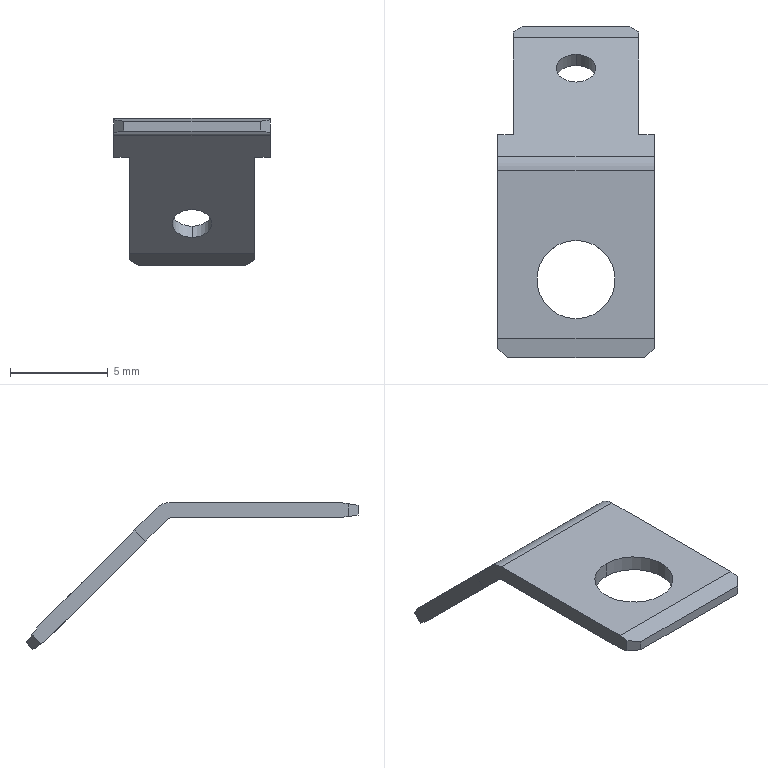Part | STEP file | DXDZ_1_1_1_1 | 1 solid | 26 faces | box 8 x 16.965 x 7.531 mm | volume 100.473 mm3 | plane 20 | cylinder 6 | commonest cylinder face diameters 2 x3 4 x2 0.4 x1
STEP:
#1=CARTESIAN_POINT('',(0.,0.,0.));
#2=DIRECTION('',(0.,0.,1.));
#3=DIRECTION('',(1.,0.,0.));
#4=AXIS2_PLACEMENT_3D('',#1,#2,#3);
#5=CARTESIAN_POINT('',(0.,0.8485,-1.98));
#6=VERTEX_POINT('',#5);
#7=CARTESIAN_POINT('',(0.,1.414,-1.414));
#8=VERTEX_POINT('',#7);
#9=CARTESIAN_POINT('',(0.,0.8485,-1.98));
#10=DIRECTION('',(0.,0.7071,0.7071));
#11=VECTOR('',#10,0.8);
#12=LINE('',#9,#11);
#13=EDGE_CURVE('',#6,#8,#12,.T.);
#14=ORIENTED_EDGE('',*,*,#13,.T.);
#15=CARTESIAN_POINT('',(0.,0.2929,-0.2929));
#16=VERTEX_POINT('',#15);
#17=CARTESIAN_POINT('',(0.,1.414,-1.414));
#18=DIRECTION('',(0.,-0.7071,0.7071));
#19=VECTOR('',#18,1.586);
#20=LINE('',#17,#19);
#21=EDGE_CURVE('',#8,#16,#20,.T.);
#22=ORIENTED_EDGE('',*,*,#21,.T.);
#23=CARTESIAN_POINT('',(0.,-0.4142,0.));
#24=VERTEX_POINT('',#23);
#25=CARTESIAN_POINT('',(0.,-0.4142,-1.));
#26=DIRECTION('',(1.,0.,0.));
#27=DIRECTION('',(0.,0.7071,0.7071));
#28=AXIS2_PLACEMENT_3D('',#25,#26,#27);
#29=CIRCLE('',#28,1.);
#30=EDGE_CURVE('',#16,#24,#29,.T.);
#31=ORIENTED_EDGE('',*,*,#30,.T.);
#32=CARTESIAN_POINT('',(0.,-9.,0.));
#33=VERTEX_POINT('',#32);
#34=CARTESIAN_POINT('',(0.,-0.4142,0.));
#35=DIRECTION('',(0.,-1.,0.));
#36=VECTOR('',#35,8.586);
#37=LINE('',#34,#36);
#38=EDGE_CURVE('',#24,#33,#37,.T.);
#39=ORIENTED_EDGE('',*,*,#38,.T.);
#40=CARTESIAN_POINT('',(0.,-9.5,-0.075));
#41=VERTEX_POINT('',#40);
#42=CARTESIAN_POINT('',(0.,-9.,0.));
#43=DIRECTION('',(0.,-0.9889,-0.1483));
#44=VECTOR('',#43,0.5056);
#45=LINE('',#42,#44);
#46=EDGE_CURVE('',#33,#41,#45,.T.);
#47=ORIENTED_EDGE('',*,*,#46,.T.);
#48=CARTESIAN_POINT('',(0.,-9.5,-0.725));
#49=VERTEX_POINT('',#48);
#50=CARTESIAN_POINT('',(0.,-9.5,-0.725));
#51=DIRECTION('',(0.,0.,1.));
#52=VECTOR('',#51,0.65);
#53=LINE('',#50,#52);
#54=EDGE_CURVE('',#49,#41,#53,.T.);
#55=ORIENTED_EDGE('',*,*,#54,.F.);
#56=CARTESIAN_POINT('',(0.,-9.,-0.8));
#57=VERTEX_POINT('',#56);
#58=CARTESIAN_POINT('',(0.,-9.5,-0.725));
#59=DIRECTION('',(0.,0.9889,-0.1483));
#60=VECTOR('',#59,0.5056);
#61=LINE('',#58,#60);
#62=EDGE_CURVE('',#49,#57,#61,.T.);
#63=ORIENTED_EDGE('',*,*,#62,.T.);
#64=CARTESIAN_POINT('',(0.,-0.4142,-0.8));
#65=VERTEX_POINT('',#64);
#66=CARTESIAN_POINT('',(0.,-9.,-0.8));
#67=DIRECTION('',(0.,1.,0.));
#68=VECTOR('',#67,8.586);
#69=LINE('',#66,#68);
#70=EDGE_CURVE('',#57,#65,#69,.T.);
#71=ORIENTED_EDGE('',*,*,#70,.T.);
#72=CARTESIAN_POINT('',(0.,-0.2728,-0.8586));
#73=VERTEX_POINT('',#72);
#74=CARTESIAN_POINT('',(0.,-0.4142,-1.));
#75=DIRECTION('',(-1.,0.,0.));
#76=DIRECTION('',(0.,0.,1.));
#77=AXIS2_PLACEMENT_3D('',#74,#75,#76);
#78=CIRCLE('',#77,0.2);
#79=EDGE_CURVE('',#65,#73,#78,.T.);
#80=ORIENTED_EDGE('',*,*,#79,.T.);
#81=CARTESIAN_POINT('',(0.,-0.2728,-0.8586));
#82=DIRECTION('',(0.,0.7071,-0.7071));
#83=VECTOR('',#82,1.586);
#84=LINE('',#81,#83);
#85=EDGE_CURVE('',#73,#6,#84,.T.);
#86=ORIENTED_EDGE('',*,*,#85,.T.);
#87=EDGE_LOOP('',(#14,#22,#31,#39,#47,#55,#63,#71,#80,#86));
#88=FACE_OUTER_BOUND('',#87,.F.);
#89=CARTESIAN_POINT('',(0.,0.,0.));
#90=DIRECTION('',(1.,0.,0.));
#91=DIRECTION('',(0.,-1.,0.));
#92=AXIS2_PLACEMENT_3D('',#89,#90,#91);
#93=PLANE('',#92);
#94=ADVANCED_FACE('',(#88),#93,.F.);
#95=ORIENTED_EDGE('',*,*,#13,.F.);
#96=CARTESIAN_POINT('',(0.8,0.8485,-1.98));
#97=VERTEX_POINT('',#96);
#98=CARTESIAN_POINT('',(0.,0.8485,-1.98));
#99=DIRECTION('',(1.,0.,0.));
#100=VECTOR('',#99,0.8);
#101=LINE('',#98,#100);
#102=EDGE_CURVE('',#6,#97,#101,.T.);
#103=ORIENTED_EDGE('',*,*,#102,.T.);
#104=CARTESIAN_POINT('',(0.8,1.414,-1.414));
#105=VERTEX_POINT('',#104);
#106=CARTESIAN_POINT('',(0.8,0.8485,-1.98));
#107=DIRECTION('',(0.,0.7071,0.7071));
#108=VECTOR('',#107,0.8);
#109=LINE('',#106,#108);
#110=EDGE_CURVE('',#97,#105,#109,.T.);
#111=ORIENTED_EDGE('',*,*,#110,.T.);
#112=CARTESIAN_POINT('',(0.,1.414,-1.414));
#113=DIRECTION('',(1.,0.,0.));
#114=VECTOR('',#113,0.8);
#115=LINE('',#112,#114);
#116=EDGE_CURVE('',#8,#105,#115,.T.);
#117=ORIENTED_EDGE('',*,*,#116,.F.);
#118=EDGE_LOOP('',(#95,#103,#111,#117));
#119=FACE_OUTER_BOUND('',#118,.F.);
#120=CARTESIAN_POINT('',(0.8,0.8485,-1.98));
#121=DIRECTION('',(0.,-0.7071,0.7071));
#122=DIRECTION('',(-1.,0.,0.));
#123=AXIS2_PLACEMENT_3D('',#120,#121,#122);
#124=PLANE('',#123);
#125=ADVANCED_FACE('',(#119),#124,.F.);
#126=CARTESIAN_POINT('',(7.2,5.798,-6.93));
#127=VERTEX_POINT('',#126);
#128=CARTESIAN_POINT('',(0.8,5.798,-6.93));
#129=VERTEX_POINT('',#128);
#130=CARTESIAN_POINT('',(7.2,5.798,-6.93));
#131=DIRECTION('',(-1.,0.,0.));
#132=VECTOR('',#131,6.4);
#133=LINE('',#130,#132);
#134=EDGE_CURVE('',#127,#129,#133,.T.);
#135=ORIENTED_EDGE('',*,*,#134,.T.);
#136=CARTESIAN_POINT('',(0.8,5.798,-6.93));
#137=DIRECTION('',(0.,-0.7071,0.7071));
#138=VECTOR('',#137,7.);
#139=LINE('',#136,#138);
#140=EDGE_CURVE('',#129,#97,#139,.T.);
#141=ORIENTED_EDGE('',*,*,#140,.T.);
#142=ORIENTED_EDGE('',*,*,#102,.F.);
#143=ORIENTED_EDGE('',*,*,#85,.F.);
#144=CARTESIAN_POINT('',(8.,-0.2728,-0.8586));
#145=VERTEX_POINT('',#144);
#146=CARTESIAN_POINT('',(8.,-0.2728,-0.8586));
#147=DIRECTION('',(-1.,0.,0.));
#148=VECTOR('',#147,8.);
#149=LINE('',#146,#148);
#150=EDGE_CURVE('',#145,#73,#149,.T.);
#151=ORIENTED_EDGE('',*,*,#150,.F.);
#152=CARTESIAN_POINT('',(8.,0.8485,-1.98));
#153=VERTEX_POINT('',#152);
#154=CARTESIAN_POINT('',(8.,0.8485,-1.98));
#155=DIRECTION('',(0.,-0.7071,0.7071));
#156=VECTOR('',#155,1.586);
#157=LINE('',#154,#156);
#158=EDGE_CURVE('',#153,#145,#157,.T.);
#159=ORIENTED_EDGE('',*,*,#158,.F.);
#160=CARTESIAN_POINT('',(7.2,0.8485,-1.98));
#161=VERTEX_POINT('',#160);
#162=CARTESIAN_POINT('',(8.,0.8485,-1.98));
#163=DIRECTION('',(-1.,0.,0.));
#164=VECTOR('',#163,0.8);
#165=LINE('',#162,#164);
#166=EDGE_CURVE('',#153,#161,#165,.T.);
#167=ORIENTED_EDGE('',*,*,#166,.T.);
#168=CARTESIAN_POINT('',(7.2,5.798,-6.93));
#169=DIRECTION('',(0.,-0.7071,0.7071));
#170=VECTOR('',#169,7.);
#171=LINE('',#168,#170);
#172=EDGE_CURVE('',#127,#161,#171,.T.);
#173=ORIENTED_EDGE('',*,*,#172,.F.);
#174=EDGE_LOOP('',(#135,#141,#142,#143,#151,#159,#167,#173));
#175=FACE_OUTER_BOUND('',#174,.F.);
#176=CARTESIAN_POINT('',(4.,3.536,-4.667));
#177=VERTEX_POINT('',#176);
#178=CARTESIAN_POINT('',(4.,4.95,-6.081));
#179=VERTEX_POINT('',#178);
#180=CARTESIAN_POINT('',(4.,4.243,-5.374));
#181=DIRECTION('',(0.,-0.7071,-0.7071));
#182=DIRECTION('',(0.,-0.7071,0.7071));
#183=AXIS2_PLACEMENT_3D('',#180,#181,#182);
#184=CIRCLE('',#183,1.);
#185=EDGE_CURVE('',#177,#179,#184,.T.);
#186=ORIENTED_EDGE('',*,*,#185,.T.);
#187=CARTESIAN_POINT('',(4.,4.243,-5.374));
#188=DIRECTION('',(0.,-0.7071,-0.7071));
#189=DIRECTION('',(0.,0.7071,-0.7071));
#190=AXIS2_PLACEMENT_3D('',#187,#188,#189);
#191=CIRCLE('',#190,1.);
#192=EDGE_CURVE('',#179,#177,#191,.T.);
#193=ORIENTED_EDGE('',*,*,#192,.T.);
#194=EDGE_LOOP('',(#186,#193));
#195=FACE_BOUND('',#194,.F.);
#196=CARTESIAN_POINT('',(0.,-0.3314,-0.8));
#197=DIRECTION('',(0.,-0.7071,-0.7071));
#198=DIRECTION('',(0.,0.7071,-0.7071));
#199=AXIS2_PLACEMENT_3D('',#196,#197,#198);
#200=PLANE('',#199);
#201=ADVANCED_FACE('',(#175,#195),#200,.T.);
#202=CARTESIAN_POINT('',(1.3,6.611,-7.531));
#203=VERTEX_POINT('',#202);
#204=CARTESIAN_POINT('',(0.8,6.205,-7.23));
#205=VERTEX_POINT('',#204);
#206=CARTESIAN_POINT('',(1.3,6.611,-7.531));
#207=DIRECTION('',(-0.7032,-0.5718,0.4226));
#208=VECTOR('',#207,0.7111);
#209=LINE('',#206,#208);
#210=EDGE_CURVE('',#203,#205,#209,.T.);
#211=ORIENTED_EDGE('',*,*,#210,.T.);
#212=CARTESIAN_POINT('',(0.8,5.798,-6.93));
#213=DIRECTION('',(0.,0.8042,-0.5944));
#214=VECTOR('',#213,0.5056);
#215=LINE('',#212,#214);
#216=EDGE_CURVE('',#129,#205,#215,.T.);
#217=ORIENTED_EDGE('',*,*,#216,.F.);
#218=ORIENTED_EDGE('',*,*,#134,.F.);
#219=CARTESIAN_POINT('',(7.2,6.205,-7.23));
#220=VERTEX_POINT('',#219);
#221=CARTESIAN_POINT('',(7.2,6.205,-7.23));
#222=DIRECTION('',(0.,-0.8042,0.5944));
#223=VECTOR('',#222,0.5056);
#224=LINE('',#221,#223);
#225=EDGE_CURVE('',#220,#127,#224,.T.);
#226=ORIENTED_EDGE('',*,*,#225,.F.);
#227=CARTESIAN_POINT('',(6.7,6.611,-7.531));
#228=VERTEX_POINT('',#227);
#229=CARTESIAN_POINT('',(7.2,6.205,-7.23));
#230=DIRECTION('',(-0.7032,0.5718,-0.4226));
#231=VECTOR('',#230,0.7111);
#232=LINE('',#229,#231);
#233=EDGE_CURVE('',#220,#228,#232,.T.);
#234=ORIENTED_EDGE('',*,*,#233,.T.);
#235=CARTESIAN_POINT('',(6.7,6.611,-7.531));
#236=DIRECTION('',(-1.,0.,0.));
#237=VECTOR('',#236,5.4);
#238=LINE('',#235,#237);
#239=EDGE_CURVE('',#228,#203,#238,.T.);
#240=ORIENTED_EDGE('',*,*,#239,.T.);
#241=EDGE_LOOP('',(#211,#217,#218,#226,#234,#240));
#242=FACE_OUTER_BOUND('',#241,.F.);
#243=CARTESIAN_POINT('',(4.,6.205,-7.23));
#244=DIRECTION('',(0.,-0.5944,-0.8042));
#245=DIRECTION('',(0.,-0.8042,0.5944));
#246=AXIS2_PLACEMENT_3D('',#243,#244,#245);
#247=PLANE('',#246);
#248=ADVANCED_FACE('',(#242),#247,.T.);
#249=CARTESIAN_POINT('',(0.8,6.664,-6.771));
#250=VERTEX_POINT('',#249);
#251=CARTESIAN_POINT('',(1.3,6.965,-7.177));
#252=VERTEX_POINT('',#251);
#253=CARTESIAN_POINT('',(0.8,6.664,-6.771));
#254=DIRECTION('',(0.7032,0.4226,-0.5718));
#255=VECTOR('',#254,0.7111);
#256=LINE('',#253,#255);
#257=EDGE_CURVE('',#250,#252,#256,.T.);
#258=ORIENTED_EDGE('',*,*,#257,.F.);
#259=CARTESIAN_POINT('',(0.8,6.205,-7.23));
#260=DIRECTION('',(0.,0.7071,0.7071));
#261=VECTOR('',#260,0.65);
#262=LINE('',#259,#261);
#263=EDGE_CURVE('',#205,#250,#262,.T.);
#264=ORIENTED_EDGE('',*,*,#263,.F.);
#265=ORIENTED_EDGE('',*,*,#210,.F.);
#266=CARTESIAN_POINT('',(1.3,6.611,-7.531));
#267=DIRECTION('',(0.,0.7071,0.7071));
#268=VECTOR('',#267,0.5);
#269=LINE('',#266,#268);
#270=EDGE_CURVE('',#203,#252,#269,.T.);
#271=ORIENTED_EDGE('',*,*,#270,.T.);
#272=EDGE_LOOP('',(#258,#264,#265,#271));
#273=FACE_OUTER_BOUND('',#272,.F.);
#274=CARTESIAN_POINT('',(1.05,6.611,-7.177));
#275=DIRECTION('',(-0.7071,0.5,-0.5));
#276=DIRECTION('',(-0.7071,-0.5,0.5));
#277=AXIS2_PLACEMENT_3D('',#274,#275,#276);
#278=PLANE('',#277);
#279=ADVANCED_FACE('',(#273),#278,.T.);
#280=CARTESIAN_POINT('',(0.8,6.364,-6.364));
#281=VERTEX_POINT('',#280);
#282=CARTESIAN_POINT('',(0.8,6.664,-6.771));
#283=DIRECTION('',(0.,-0.5944,0.8042));
#284=VECTOR('',#283,0.5056);
#285=LINE('',#282,#284);
#286=EDGE_CURVE('',#250,#281,#285,.T.);
#287=ORIENTED_EDGE('',*,*,#286,.F.);
#288=ORIENTED_EDGE('',*,*,#257,.T.);
#289=CARTESIAN_POINT('',(6.7,6.965,-7.177));
#290=VERTEX_POINT('',#289);
#291=CARTESIAN_POINT('',(6.7,6.965,-7.177));
#292=DIRECTION('',(-1.,0.,0.));
#293=VECTOR('',#292,5.4);
#294=LINE('',#291,#293);
#295=EDGE_CURVE('',#290,#252,#294,.T.);
#296=ORIENTED_EDGE('',*,*,#295,.F.);
#297=CARTESIAN_POINT('',(7.2,6.664,-6.771));
#298=VERTEX_POINT('',#297);
#299=CARTESIAN_POINT('',(6.7,6.965,-7.177));
#300=DIRECTION('',(0.7032,-0.4226,0.5718));
#301=VECTOR('',#300,0.7111);
#302=LINE('',#299,#301);
#303=EDGE_CURVE('',#290,#298,#302,.T.);
#304=ORIENTED_EDGE('',*,*,#303,.T.);
#305=CARTESIAN_POINT('',(7.2,6.364,-6.364));
#306=VERTEX_POINT('',#305);
#307=CARTESIAN_POINT('',(7.2,6.364,-6.364));
#308=DIRECTION('',(0.,0.5944,-0.8042));
#309=VECTOR('',#308,0.5056);
#310=LINE('',#307,#309);
#311=EDGE_CURVE('',#306,#298,#310,.T.);
#312=ORIENTED_EDGE('',*,*,#311,.F.);
#313=CARTESIAN_POINT('',(7.2,6.364,-6.364));
#314=DIRECTION('',(-1.,0.,0.));
#315=VECTOR('',#314,6.4);
#316=LINE('',#313,#315);
#317=EDGE_CURVE('',#306,#281,#316,.T.);
#318=ORIENTED_EDGE('',*,*,#317,.T.);
#319=EDGE_LOOP('',(#287,#288,#296,#304,#312,#318));
#320=FACE_OUTER_BOUND('',#319,.F.);
#321=CARTESIAN_POINT('',(4.,6.664,-6.771));
#322=DIRECTION('',(0.,0.8042,0.5944));
#323=DIRECTION('',(0.,0.5944,-0.8042));
#324=AXIS2_PLACEMENT_3D('',#321,#322,#323);
#325=PLANE('',#324);
#326=ADVANCED_FACE('',(#320),#325,.T.);
#327=ORIENTED_EDGE('',*,*,#286,.T.);
#328=CARTESIAN_POINT('',(0.8,6.364,-6.364));
#329=DIRECTION('',(0.,-0.7071,0.7071));
#330=VECTOR('',#329,7.);
#331=LINE('',#328,#330);
#332=EDGE_CURVE('',#281,#105,#331,.T.);
#333=ORIENTED_EDGE('',*,*,#332,.T.);
#334=ORIENTED_EDGE('',*,*,#110,.F.);
#335=ORIENTED_EDGE('',*,*,#140,.F.);
#336=ORIENTED_EDGE('',*,*,#216,.T.);
#337=ORIENTED_EDGE('',*,*,#263,.T.);
#338=EDGE_LOOP('',(#327,#333,#334,#335,#336,#337));
#339=FACE_OUTER_BOUND('',#338,.F.);
#340=CARTESIAN_POINT('',(0.8,6.505,-7.637));
#341=DIRECTION('',(1.,0.,0.));
#342=DIRECTION('',(0.,-0.7071,0.7071));
#343=AXIS2_PLACEMENT_3D('',#340,#341,#342);
#344=PLANE('',#343);
#345=ADVANCED_FACE('',(#339),#344,.F.);
#346=ORIENTED_EDGE('',*,*,#317,.F.);
#347=CARTESIAN_POINT('',(7.2,1.414,-1.414));
#348=VERTEX_POINT('',#347);
#349=CARTESIAN_POINT('',(7.2,6.364,-6.364));
#350=DIRECTION('',(0.,-0.7071,0.7071));
#351=VECTOR('',#350,7.);
#352=LINE('',#349,#351);
#353=EDGE_CURVE('',#306,#348,#352,.T.);
#354=ORIENTED_EDGE('',*,*,#353,.T.);
#355=CARTESIAN_POINT('',(8.,1.414,-1.414));
#356=VERTEX_POINT('',#355);
#357=CARTESIAN_POINT('',(8.,1.414,-1.414));
#358=DIRECTION('',(-1.,0.,0.));
#359=VECTOR('',#358,0.8);
#360=LINE('',#357,#359);
#361=EDGE_CURVE('',#356,#348,#360,.T.);
#362=ORIENTED_EDGE('',*,*,#361,.F.);
#363=CARTESIAN_POINT('',(8.,0.2929,-0.2929));
#364=VERTEX_POINT('',#363);
#365=CARTESIAN_POINT('',(8.,0.2929,-0.2929));
#366=DIRECTION('',(0.,0.7071,-0.7071));
#367=VECTOR('',#366,1.586);
#368=LINE('',#365,#367);
#369=EDGE_CURVE('',#364,#356,#368,.T.);
#370=ORIENTED_EDGE('',*,*,#369,.F.);
#371=CARTESIAN_POINT('',(0.,0.2929,-0.2929));
#372=DIRECTION('',(1.,0.,0.));
#373=VECTOR('',#372,8.);
#374=LINE('',#371,#373);
#375=EDGE_CURVE('',#16,#364,#374,.T.);
#376=ORIENTED_EDGE('',*,*,#375,.F.);
#377=ORIENTED_EDGE('',*,*,#21,.F.);
#378=ORIENTED_EDGE('',*,*,#116,.T.);
#379=ORIENTED_EDGE('',*,*,#332,.F.);
#380=EDGE_LOOP('',(#346,#354,#362,#370,#376,#377,#378,#379));
#381=FACE_OUTER_BOUND('',#380,.F.);
#382=CARTESIAN_POINT('',(4.,5.515,-5.515));
#383=VERTEX_POINT('',#382);
#384=CARTESIAN_POINT('',(4.,4.101,-4.101));
#385=VERTEX_POINT('',#384);
#386=CARTESIAN_POINT('',(4.,4.808,-4.808));
#387=DIRECTION('',(0.,0.7071,0.7071));
#388=DIRECTION('',(0.,0.7071,-0.7071));
#389=AXIS2_PLACEMENT_3D('',#386,#387,#388);
#390=CIRCLE('',#389,1.);
#391=EDGE_CURVE('',#383,#385,#390,.T.);
#392=ORIENTED_EDGE('',*,*,#391,.T.);
#393=CARTESIAN_POINT('',(4.,4.808,-4.808));
#394=DIRECTION('',(0.,0.7071,0.7071));
#395=DIRECTION('',(0.,-0.7071,0.7071));
#396=AXIS2_PLACEMENT_3D('',#393,#394,#395);
#397=CIRCLE('',#396,1.);
#398=EDGE_CURVE('',#385,#383,#397,.T.);
#399=ORIENTED_EDGE('',*,*,#398,.T.);
#400=EDGE_LOOP('',(#392,#399));
#401=FACE_BOUND('',#400,.F.);
#402=CARTESIAN_POINT('',(0.,7.071,-7.071));
#403=DIRECTION('',(0.,0.7071,0.7071));
#404=DIRECTION('',(0.,-0.7071,0.7071));
#405=AXIS2_PLACEMENT_3D('',#402,#403,#404);
#406=PLANE('',#405);
#407=ADVANCED_FACE('',(#381,#401),#406,.T.);
#408=ORIENTED_EDGE('',*,*,#311,.T.);
#409=CARTESIAN_POINT('',(7.2,6.664,-6.771));
#410=DIRECTION('',(0.,-0.7071,-0.7071));
#411=VECTOR('',#410,0.65);
#412=LINE('',#409,#411);
#413=EDGE_CURVE('',#298,#220,#412,.T.);
#414=ORIENTED_EDGE('',*,*,#413,.T.);
#415=ORIENTED_EDGE('',*,*,#225,.T.);
#416=ORIENTED_EDGE('',*,*,#172,.T.);
#417=CARTESIAN_POINT('',(7.2,0.8485,-1.98));
#418=DIRECTION('',(0.,0.7071,0.7071));
#419=VECTOR('',#418,0.8);
#420=LINE('',#417,#419);
#421=EDGE_CURVE('',#161,#348,#420,.T.);
#422=ORIENTED_EDGE('',*,*,#421,.T.);
#423=ORIENTED_EDGE('',*,*,#353,.F.);
#424=EDGE_LOOP('',(#408,#414,#415,#416,#422,#423));
#425=FACE_OUTER_BOUND('',#424,.F.);
#426=CARTESIAN_POINT('',(7.2,0.8485,-1.98));
#427=DIRECTION('',(-1.,0.,0.));
#428=DIRECTION('',(0.,0.7071,-0.7071));
#429=AXIS2_PLACEMENT_3D('',#426,#427,#428);
#430=PLANE('',#429);
#431=ADVANCED_FACE('',(#425),#430,.F.);
#432=ORIENTED_EDGE('',*,*,#303,.F.);
#433=CARTESIAN_POINT('',(6.7,6.965,-7.177));
#434=DIRECTION('',(0.,-0.7071,-0.7071));
#435=VECTOR('',#434,0.5);
#436=LINE('',#433,#435);
#437=EDGE_CURVE('',#290,#228,#436,.T.);
#438=ORIENTED_EDGE('',*,*,#437,.T.);
#439=ORIENTED_EDGE('',*,*,#233,.F.);
#440=ORIENTED_EDGE('',*,*,#413,.F.);
#441=EDGE_LOOP('',(#432,#438,#439,#440));
#442=FACE_OUTER_BOUND('',#441,.F.);
#443=CARTESIAN_POINT('',(6.95,6.611,-7.177));
#444=DIRECTION('',(0.7071,0.5,-0.5));
#445=DIRECTION('',(0.7071,-0.5,0.5));
#446=AXIS2_PLACEMENT_3D('',#443,#444,#445);
#447=PLANE('',#446);
#448=ADVANCED_FACE('',(#442),#447,.T.);
#449=ORIENTED_EDGE('',*,*,#295,.T.);
#450=ORIENTED_EDGE('',*,*,#270,.F.);
#451=ORIENTED_EDGE('',*,*,#239,.F.);
#452=ORIENTED_EDGE('',*,*,#437,.F.);
#453=EDGE_LOOP('',(#449,#450,#451,#452));
#454=FACE_OUTER_BOUND('',#453,.F.);
#455=CARTESIAN_POINT('',(0.,6.505,-7.637));
#456=DIRECTION('',(0.,0.7071,-0.7071));
#457=DIRECTION('',(0.,0.7071,0.7071));
#458=AXIS2_PLACEMENT_3D('',#455,#456,#457);
#459=PLANE('',#458);
#460=ADVANCED_FACE('',(#454),#459,.T.);
#461=CARTESIAN_POINT('',(8.,1.414,-1.414));
#462=DIRECTION('',(0.,-0.7071,-0.7071));
#463=VECTOR('',#462,0.8);
#464=LINE('',#461,#463);
#465=EDGE_CURVE('',#356,#153,#464,.T.);
#466=ORIENTED_EDGE('',*,*,#465,.F.);
#467=ORIENTED_EDGE('',*,*,#361,.T.);
#468=ORIENTED_EDGE('',*,*,#421,.F.);
#469=ORIENTED_EDGE('',*,*,#166,.F.);
#470=EDGE_LOOP('',(#466,#467,#468,#469));
#471=FACE_OUTER_BOUND('',#470,.F.);
#472=CARTESIAN_POINT('',(8.,0.8485,-1.98));
#473=DIRECTION('',(0.,-0.7071,0.7071));
#474=DIRECTION('',(-1.,0.,0.));
#475=AXIS2_PLACEMENT_3D('',#472,#473,#474);
#476=PLANE('',#475);
#477=ADVANCED_FACE('',(#471),#476,.F.);
#478=ORIENTED_EDGE('',*,*,#465,.T.);
#479=ORIENTED_EDGE('',*,*,#158,.T.);
#480=CARTESIAN_POINT('',(8.,-0.4142,-0.8));
#481=VERTEX_POINT('',#480);
#482=CARTESIAN_POINT('',(8.,-0.4142,-1.));
#483=DIRECTION('',(1.,0.,0.));
#484=DIRECTION('',(0.,0.7071,0.7071));
#485=AXIS2_PLACEMENT_3D('',#482,#483,#484);
#486=CIRCLE('',#485,0.2);
#487=EDGE_CURVE('',#145,#481,#486,.T.);
#488=ORIENTED_EDGE('',*,*,#487,.T.);
#489=CARTESIAN_POINT('',(8.,-9.,-0.8));
#490=VERTEX_POINT('',#489);
#491=CARTESIAN_POINT('',(8.,-9.,-0.8));
#492=DIRECTION('',(0.,1.,0.));
#493=VECTOR('',#492,8.586);
#494=LINE('',#491,#493);
#495=EDGE_CURVE('',#490,#481,#494,.T.);
#496=ORIENTED_EDGE('',*,*,#495,.F.);
#497=CARTESIAN_POINT('',(8.,-9.5,-0.725));
#498=VERTEX_POINT('',#497);
#499=CARTESIAN_POINT('',(8.,-9.,-0.8));
#500=DIRECTION('',(0.,-0.9889,0.1483));
#501=VECTOR('',#500,0.5056);
#502=LINE('',#499,#501);
#503=EDGE_CURVE('',#490,#498,#502,.T.);
#504=ORIENTED_EDGE('',*,*,#503,.T.);
#505=CARTESIAN_POINT('',(8.,-9.5,-0.075));
#506=VERTEX_POINT('',#505);
#507=CARTESIAN_POINT('',(8.,-9.5,-0.075));
#508=DIRECTION('',(0.,0.,-1.));
#509=VECTOR('',#508,0.65);
#510=LINE('',#507,#509);
#511=EDGE_CURVE('',#506,#498,#510,.T.);
#512=ORIENTED_EDGE('',*,*,#511,.F.);
#513=CARTESIAN_POINT('',(8.,-9.,0.));
#514=VERTEX_POINT('',#513);
#515=CARTESIAN_POINT('',(8.,-9.5,-0.075));
#516=DIRECTION('',(0.,0.9889,0.1483));
#517=VECTOR('',#516,0.5056);
#518=LINE('',#515,#517);
#519=EDGE_CURVE('',#506,#514,#518,.T.);
#520=ORIENTED_EDGE('',*,*,#519,.T.);
#521=CARTESIAN_POINT('',(8.,-0.4142,0.));
#522=VERTEX_POINT('',#521);
#523=CARTESIAN_POINT('',(8.,-0.4142,0.));
#524=DIRECTION('',(0.,-1.,0.));
#525=VECTOR('',#524,8.586);
#526=LINE('',#523,#525);
#527=EDGE_CURVE('',#522,#514,#526,.T.);
#528=ORIENTED_EDGE('',*,*,#527,.F.);
#529=CARTESIAN_POINT('',(8.,-0.4142,-1.));
#530=DIRECTION('',(-1.,0.,0.));
#531=DIRECTION('',(0.,0.,1.));
#532=AXIS2_PLACEMENT_3D('',#529,#530,#531);
#533=CIRCLE('',#532,1.);
#534=EDGE_CURVE('',#522,#364,#533,.T.);
#535=ORIENTED_EDGE('',*,*,#534,.T.);
#536=ORIENTED_EDGE('',*,*,#369,.T.);
#537=EDGE_LOOP('',(#478,#479,#488,#496,#504,#512,#520,#528,#535,#536));
#538=FACE_OUTER_BOUND('',#537,.F.);
#539=CARTESIAN_POINT('',(8.,0.,0.));
#540=DIRECTION('',(1.,0.,0.));
#541=DIRECTION('',(0.,-1.,0.));
#542=AXIS2_PLACEMENT_3D('',#539,#540,#541);
#543=PLANE('',#542);
#544=ADVANCED_FACE('',(#538),#543,.T.);
#545=ORIENTED_EDGE('',*,*,#150,.T.);
#546=ORIENTED_EDGE('',*,*,#79,.F.);
#547=CARTESIAN_POINT('',(0.,-0.4142,-0.8));
#548=DIRECTION('',(1.,0.,0.));
#549=VECTOR('',#548,8.);
#550=LINE('',#547,#549);
#551=EDGE_CURVE('',#65,#481,#550,.T.);
#552=ORIENTED_EDGE('',*,*,#551,.T.);
#553=ORIENTED_EDGE('',*,*,#487,.F.);
#554=EDGE_LOOP('',(#545,#546,#552,#553));
#555=FACE_OUTER_BOUND('',#554,.F.);
#556=CARTESIAN_POINT('',(-10.429,-0.4142,-1.));
#557=DIRECTION('',(1.,0.,0.));
#558=DIRECTION('',(0.,0.7071,0.7071));
#559=AXIS2_PLACEMENT_3D('',#556,#557,#558);
#560=CYLINDRICAL_SURFACE('',#559,0.2);
#561=ADVANCED_FACE('',(#555),#560,.F.);
#562=CARTESIAN_POINT('',(8.,-9.,-0.8));
#563=DIRECTION('',(-1.,0.,0.));
#564=VECTOR('',#563,8.);
#565=LINE('',#562,#564);
#566=EDGE_CURVE('',#490,#57,#565,.T.);
#567=ORIENTED_EDGE('',*,*,#566,.F.);
#568=ORIENTED_EDGE('',*,*,#495,.T.);
#569=ORIENTED_EDGE('',*,*,#551,.F.);
#570=ORIENTED_EDGE('',*,*,#70,.F.);
#571=EDGE_LOOP('',(#567,#568,#569,#570));
#572=FACE_OUTER_BOUND('',#571,.F.);
#573=CARTESIAN_POINT('',(4.,-8.,-0.8));
#574=VERTEX_POINT('',#573);
#575=CARTESIAN_POINT('',(4.,-4.,-0.8));
#576=VERTEX_POINT('',#575);
#577=CARTESIAN_POINT('',(4.,-6.,-0.8));
#578=DIRECTION('',(0.,0.,-1.));
#579=DIRECTION('',(0.,-1.,0.));
#580=AXIS2_PLACEMENT_3D('',#577,#578,#579);
#581=CIRCLE('',#580,2.);
#582=EDGE_CURVE('',#574,#576,#581,.T.);
#583=ORIENTED_EDGE('',*,*,#582,.T.);
#584=CARTESIAN_POINT('',(4.,-6.,-0.8));
#585=DIRECTION('',(0.,0.,-1.));
#586=DIRECTION('',(0.,1.,0.));
#587=AXIS2_PLACEMENT_3D('',#584,#585,#586);
#588=CIRCLE('',#587,2.);
#589=EDGE_CURVE('',#576,#574,#588,.T.);
#590=ORIENTED_EDGE('',*,*,#589,.T.);
#591=EDGE_LOOP('',(#583,#590));
#592=FACE_BOUND('',#591,.F.);
#593=CARTESIAN_POINT('',(0.,-10.,-0.8));
#594=DIRECTION('',(0.,0.,-1.));
#595=DIRECTION('',(0.,1.,0.));
#596=AXIS2_PLACEMENT_3D('',#593,#594,#595);
#597=PLANE('',#596);
#598=ADVANCED_FACE('',(#572,#592),#597,.T.);
#599=ORIENTED_EDGE('',*,*,#62,.F.);
#600=CARTESIAN_POINT('',(0.5,-10.,-0.65));
#601=VERTEX_POINT('',#600);
#602=CARTESIAN_POINT('',(0.,-9.5,-0.725));
#603=DIRECTION('',(0.7032,-0.7032,0.1055));
#604=VECTOR('',#603,0.7111);
#605=LINE('',#602,#604);
#606=EDGE_CURVE('',#49,#601,#605,.T.);
#607=ORIENTED_EDGE('',*,*,#606,.T.);
#608=CARTESIAN_POINT('',(7.5,-10.,-0.65));
#609=VERTEX_POINT('',#608);
#610=CARTESIAN_POINT('',(7.5,-10.,-0.65));
#611=DIRECTION('',(-1.,0.,0.));
#612=VECTOR('',#611,7.);
#613=LINE('',#610,#612);
#614=EDGE_CURVE('',#609,#601,#613,.T.);
#615=ORIENTED_EDGE('',*,*,#614,.F.);
#616=CARTESIAN_POINT('',(7.5,-10.,-0.65));
#617=DIRECTION('',(0.7032,0.7032,-0.1055));
#618=VECTOR('',#617,0.7111);
#619=LINE('',#616,#618);
#620=EDGE_CURVE('',#609,#498,#619,.T.);
#621=ORIENTED_EDGE('',*,*,#620,.T.);
#622=ORIENTED_EDGE('',*,*,#503,.F.);
#623=ORIENTED_EDGE('',*,*,#566,.T.);
#624=EDGE_LOOP('',(#599,#607,#615,#621,#622,#623));
#625=FACE_OUTER_BOUND('',#624,.F.);
#626=CARTESIAN_POINT('',(4.,-9.5,-0.725));
#627=DIRECTION('',(0.,-0.1483,-0.9889));
#628=DIRECTION('',(0.,-0.9889,0.1483));
#629=AXIS2_PLACEMENT_3D('',#626,#627,#628);
#630=PLANE('',#629);
#631=ADVANCED_FACE('',(#625),#630,.T.);
#632=CARTESIAN_POINT('',(0.5,-10.,-0.15));
#633=VERTEX_POINT('',#632);
#634=CARTESIAN_POINT('',(0.5,-10.,-0.15));
#635=DIRECTION('',(-0.7032,0.7032,0.1055));
#636=VECTOR('',#635,0.7111);
#637=LINE('',#634,#636);
#638=EDGE_CURVE('',#633,#41,#637,.T.);
#639=ORIENTED_EDGE('',*,*,#638,.F.);
#640=CARTESIAN_POINT('',(0.5,-10.,-0.65));
#641=DIRECTION('',(0.,0.,1.));
#642=VECTOR('',#641,0.5);
#643=LINE('',#640,#642);
#644=EDGE_CURVE('',#601,#633,#643,.T.);
#645=ORIENTED_EDGE('',*,*,#644,.F.);
#646=ORIENTED_EDGE('',*,*,#606,.F.);
#647=ORIENTED_EDGE('',*,*,#54,.T.);
#648=EDGE_LOOP('',(#639,#645,#646,#647));
#649=FACE_OUTER_BOUND('',#648,.F.);
#650=CARTESIAN_POINT('',(0.25,-9.75,-0.4));
#651=DIRECTION('',(-0.7071,-0.7071,0.));
#652=DIRECTION('',(0.7071,-0.7071,0.));
#653=AXIS2_PLACEMENT_3D('',#650,#651,#652);
#654=PLANE('',#653);
#655=ADVANCED_FACE('',(#649),#654,.T.);
#656=ORIENTED_EDGE('',*,*,#638,.T.);
#657=ORIENTED_EDGE('',*,*,#46,.F.);
#658=CARTESIAN_POINT('',(8.,-9.,0.));
#659=DIRECTION('',(-1.,0.,0.));
#660=VECTOR('',#659,8.);
#661=LINE('',#658,#660);
#662=EDGE_CURVE('',#514,#33,#661,.T.);
#663=ORIENTED_EDGE('',*,*,#662,.F.);
#664=ORIENTED_EDGE('',*,*,#519,.F.);
#665=CARTESIAN_POINT('',(7.5,-10.,-0.15));
#666=VERTEX_POINT('',#665);
#667=CARTESIAN_POINT('',(8.,-9.5,-0.075));
#668=DIRECTION('',(-0.7032,-0.7032,-0.1055));
#669=VECTOR('',#668,0.7111);
#670=LINE('',#667,#669);
#671=EDGE_CURVE('',#506,#666,#670,.T.);
#672=ORIENTED_EDGE('',*,*,#671,.T.);
#673=CARTESIAN_POINT('',(7.5,-10.,-0.15));
#674=DIRECTION('',(-1.,0.,0.));
#675=VECTOR('',#674,7.);
#676=LINE('',#673,#675);
#677=EDGE_CURVE('',#666,#633,#676,.T.);
#678=ORIENTED_EDGE('',*,*,#677,.T.);
#679=EDGE_LOOP('',(#656,#657,#663,#664,#672,#678));
#680=FACE_OUTER_BOUND('',#679,.F.);
#681=CARTESIAN_POINT('',(4.,-9.5,-0.075));
#682=DIRECTION('',(0.,-0.1483,0.9889));
#683=DIRECTION('',(0.,0.9889,0.1483));
#684=AXIS2_PLACEMENT_3D('',#681,#682,#683);
#685=PLANE('',#684);
#686=ADVANCED_FACE('',(#680),#685,.T.);
#687=ORIENTED_EDGE('',*,*,#662,.T.);
#688=ORIENTED_EDGE('',*,*,#38,.F.);
#689=CARTESIAN_POINT('',(8.,-0.4142,0.));
#690=DIRECTION('',(-1.,0.,0.));
#691=VECTOR('',#690,8.);
#692=LINE('',#689,#691);
#693=EDGE_CURVE('',#522,#24,#692,.T.);
#694=ORIENTED_EDGE('',*,*,#693,.F.);
#695=ORIENTED_EDGE('',*,*,#527,.T.);
#696=EDGE_LOOP('',(#687,#688,#694,#695));
#697=FACE_OUTER_BOUND('',#696,.F.);
#698=CARTESIAN_POINT('',(4.,-4.,0.));
#699=VERTEX_POINT('',#698);
#700=CARTESIAN_POINT('',(4.,-8.,0.));
#701=VERTEX_POINT('',#700);
#702=CARTESIAN_POINT('',(4.,-6.,0.));
#703=DIRECTION('',(0.,0.,1.));
#704=DIRECTION('',(0.,1.,0.));
#705=AXIS2_PLACEMENT_3D('',#702,#703,#704);
#706=CIRCLE('',#705,2.);
#707=EDGE_CURVE('',#699,#701,#706,.T.);
#708=ORIENTED_EDGE('',*,*,#707,.T.);
#709=CARTESIAN_POINT('',(4.,-6.,0.));
#710=DIRECTION('',(0.,0.,1.));
#711=DIRECTION('',(0.,-1.,0.));
#712=AXIS2_PLACEMENT_3D('',#709,#710,#711);
#713=CIRCLE('',#712,2.);
#714=EDGE_CURVE('',#701,#699,#713,.T.);
#715=ORIENTED_EDGE('',*,*,#714,.T.);
#716=EDGE_LOOP('',(#708,#715));
#717=FACE_BOUND('',#716,.F.);
#718=CARTESIAN_POINT('',(0.,0.,0.));
#719=DIRECTION('',(0.,0.,1.));
#720=DIRECTION('',(0.,-1.,0.));
#721=AXIS2_PLACEMENT_3D('',#718,#719,#720);
#722=PLANE('',#721);
#723=ADVANCED_FACE('',(#697,#717),#722,.T.);
#724=ORIENTED_EDGE('',*,*,#30,.F.);
#725=ORIENTED_EDGE('',*,*,#375,.T.);
#726=ORIENTED_EDGE('',*,*,#534,.F.);
#727=ORIENTED_EDGE('',*,*,#693,.T.);
#728=EDGE_LOOP('',(#724,#725,#726,#727));
#729=FACE_OUTER_BOUND('',#728,.F.);
#730=CARTESIAN_POINT('',(18.429,-0.4142,-1.));
#731=DIRECTION('',(-1.,0.,0.));
#732=DIRECTION('',(0.,0.,1.));
#733=AXIS2_PLACEMENT_3D('',#730,#731,#732);
#734=CYLINDRICAL_SURFACE('',#733,1.);
#735=ADVANCED_FACE('',(#729),#734,.T.);
#736=ORIENTED_EDGE('',*,*,#707,.F.);
#737=CARTESIAN_POINT('',(4.,-4.,-0.8));
#738=DIRECTION('',(0.,0.,1.));
#739=VECTOR('',#738,0.8);
#740=LINE('',#737,#739);
#741=EDGE_CURVE('',#576,#699,#740,.T.);
#742=ORIENTED_EDGE('',*,*,#741,.F.);
#743=ORIENTED_EDGE('',*,*,#582,.F.);
#744=CARTESIAN_POINT('',(4.,-8.,-0.8));
#745=DIRECTION('',(0.,0.,1.));
#746=VECTOR('',#745,0.8);
#747=LINE('',#744,#746);
#748=EDGE_CURVE('',#574,#701,#747,.T.);
#749=ORIENTED_EDGE('',*,*,#748,.T.);
#750=EDGE_LOOP('',(#736,#742,#743,#749));
#751=FACE_OUTER_BOUND('',#750,.F.);
#752=CARTESIAN_POINT('',(4.,-6.,-0.8));
#753=DIRECTION('',(0.,0.,-1.));
#754=DIRECTION('',(0.,-1.,0.));
#755=AXIS2_PLACEMENT_3D('',#752,#753,#754);
#756=CYLINDRICAL_SURFACE('',#755,2.);
#757=ADVANCED_FACE('',(#751),#756,.F.);
#758=ORIENTED_EDGE('',*,*,#714,.F.);
#759=ORIENTED_EDGE('',*,*,#748,.F.);
#760=ORIENTED_EDGE('',*,*,#589,.F.);
#761=ORIENTED_EDGE('',*,*,#741,.T.);
#762=EDGE_LOOP('',(#758,#759,#760,#761));
#763=FACE_OUTER_BOUND('',#762,.F.);
#764=CARTESIAN_POINT('',(4.,-6.,-0.8));
#765=DIRECTION('',(0.,0.,-1.));
#766=DIRECTION('',(0.,-1.,0.));
#767=AXIS2_PLACEMENT_3D('',#764,#765,#766);
#768=CYLINDRICAL_SURFACE('',#767,2.);
#769=ADVANCED_FACE('',(#763),#768,.F.);
#770=ORIENTED_EDGE('',*,*,#671,.F.);
#771=ORIENTED_EDGE('',*,*,#511,.T.);
#772=ORIENTED_EDGE('',*,*,#620,.F.);
#773=CARTESIAN_POINT('',(7.5,-10.,-0.15));
#774=DIRECTION('',(0.,0.,-1.));
#775=VECTOR('',#774,0.5);
#776=LINE('',#773,#775);
#777=EDGE_CURVE('',#666,#609,#776,.T.);
#778=ORIENTED_EDGE('',*,*,#777,.F.);
#779=EDGE_LOOP('',(#770,#771,#772,#778));
#780=FACE_OUTER_BOUND('',#779,.F.);
#781=CARTESIAN_POINT('',(7.75,-9.75,-0.4));
#782=DIRECTION('',(0.7071,-0.7071,0.));
#783=DIRECTION('',(-0.7071,-0.7071,0.));
#784=AXIS2_PLACEMENT_3D('',#781,#782,#783);
#785=PLANE('',#784);
#786=ADVANCED_FACE('',(#780),#785,.T.);
#787=ORIENTED_EDGE('',*,*,#677,.F.);
#788=ORIENTED_EDGE('',*,*,#777,.T.);
#789=ORIENTED_EDGE('',*,*,#614,.T.);
#790=ORIENTED_EDGE('',*,*,#644,.T.);
#791=EDGE_LOOP('',(#787,#788,#789,#790));
#792=FACE_OUTER_BOUND('',#791,.F.);
#793=CARTESIAN_POINT('',(0.,-10.,0.));
#794=DIRECTION('',(0.,-1.,0.));
#795=DIRECTION('',(0.,0.,-1.));
#796=AXIS2_PLACEMENT_3D('',#793,#794,#795);
#797=PLANE('',#796);
#798=ADVANCED_FACE('',(#792),#797,.T.);
#799=ORIENTED_EDGE('',*,*,#185,.F.);
#800=CARTESIAN_POINT('',(4.,3.536,-4.667));
#801=DIRECTION('',(0.,0.7071,0.7071));
#802=VECTOR('',#801,0.8);
#803=LINE('',#800,#802);
#804=EDGE_CURVE('',#177,#385,#803,.T.);
#805=ORIENTED_EDGE('',*,*,#804,.T.);
#806=ORIENTED_EDGE('',*,*,#391,.F.);
#807=CARTESIAN_POINT('',(4.,4.95,-6.081));
#808=DIRECTION('',(0.,0.7071,0.7071));
#809=VECTOR('',#808,0.8);
#810=LINE('',#807,#809);
#811=EDGE_CURVE('',#179,#383,#810,.T.);
#812=ORIENTED_EDGE('',*,*,#811,.F.);
#813=EDGE_LOOP('',(#799,#805,#806,#812));
#814=FACE_OUTER_BOUND('',#813,.F.);
#815=CARTESIAN_POINT('',(4.,4.243,-5.374));
#816=DIRECTION('',(0.,-0.7071,-0.7071));
#817=DIRECTION('',(0.,-0.7071,0.7071));
#818=AXIS2_PLACEMENT_3D('',#815,#816,#817);
#819=CYLINDRICAL_SURFACE('',#818,1.);
#820=ADVANCED_FACE('',(#814),#819,.F.);
#821=ORIENTED_EDGE('',*,*,#192,.F.);
#822=ORIENTED_EDGE('',*,*,#811,.T.);
#823=ORIENTED_EDGE('',*,*,#398,.F.);
#824=ORIENTED_EDGE('',*,*,#804,.F.);
#825=EDGE_LOOP('',(#821,#822,#823,#824));
#826=FACE_OUTER_BOUND('',#825,.F.);
#827=CARTESIAN_POINT('',(4.,4.243,-5.374));
#828=DIRECTION('',(0.,-0.7071,-0.7071));
#829=DIRECTION('',(0.,-0.7071,0.7071));
#830=AXIS2_PLACEMENT_3D('',#827,#828,#829);
#831=CYLINDRICAL_SURFACE('',#830,1.);
#832=ADVANCED_FACE('',(#826),#831,.F.);
#833=CLOSED_SHELL('',(#94,#125,#201,#248,#279,#326,#345,#407,#431,#448,#460,#477,#544,#561,#598,#631,#655,#686,#723,#735,#757,#769,#786,#798,#820,#832));
#834=MANIFOLD_SOLID_BREP('',#833);
#835=(LENGTH_UNIT()NAMED_UNIT(*)SI_UNIT(.MILLI.,.METRE.));
#836=UNCERTAINTY_MEASURE_WITH_UNIT(LENGTH_MEASURE(0.002028),#835,'','');
#837=(NAMED_UNIT(*)PLANE_ANGLE_UNIT()SI_UNIT($,.RADIAN.));
#838=PLANE_ANGLE_MEASURE_WITH_UNIT(PLANE_ANGLE_MEASURE(0.01745),#837);
#839=(CONVERSION_BASED_UNIT('DEGREE',#838)NAMED_UNIT(*)PLANE_ANGLE_UNIT());
#840=(NAMED_UNIT(*)SI_UNIT($,.STERADIAN.)SOLID_ANGLE_UNIT());
#841=(GEOMETRIC_REPRESENTATION_CONTEXT(3)GLOBAL_UNCERTAINTY_ASSIGNED_CONTEXT((#836))GLOBAL_UNIT_ASSIGNED_CONTEXT((#835,#839,#840))REPRESENTATION_CONTEXT('',''));
#842=ADVANCED_BREP_SHAPE_REPRESENTATION('',(#4,#834),#841);